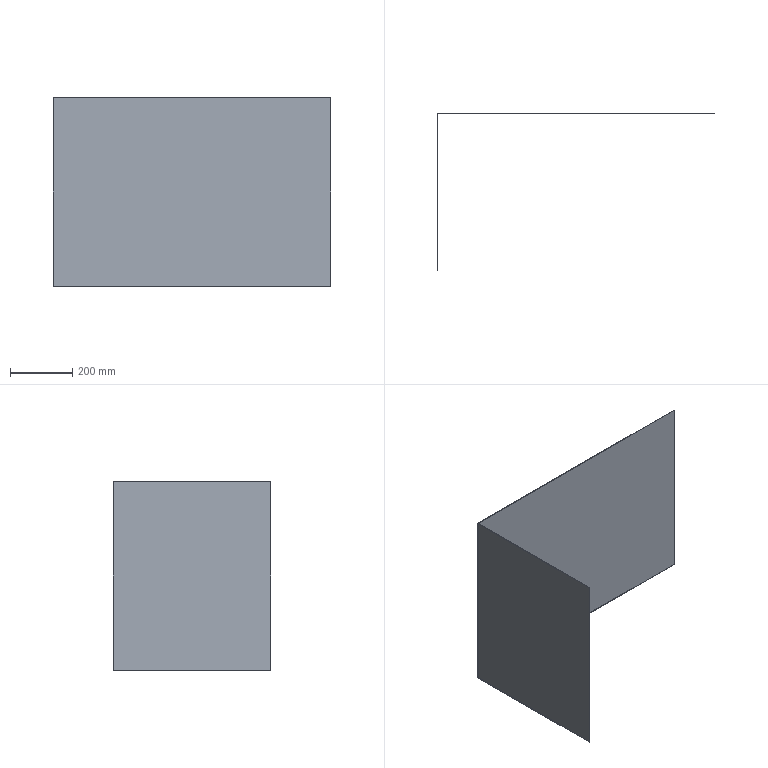Part | STEP file | zhi | 1 solid | 9 faces | box 891 x 505.5 x 606 mm | volume 845626 mm3 | plane 8 | cylinder 1 | commonest cylinder face diameters 1.2 x1
STEP:
#1=CARTESIAN_POINT('',(0.,0.,0.));
#2=DIRECTION('',(0.,0.,1.));
#3=DIRECTION('',(1.,0.,0.));
#4=AXIS2_PLACEMENT_3D('',#1,#2,#3);
#5=CARTESIAN_POINT('',(445.,-0.5,303.));
#6=VERTEX_POINT('',#5);
#7=CARTESIAN_POINT('',(445.,-0.5,-303.));
#8=VERTEX_POINT('',#7);
#9=CARTESIAN_POINT('',(445.,-0.5,-303.));
#10=DIRECTION('',(0.,0.,-1.));
#11=VECTOR('',#10,1.);
#12=LINE('',#9,#11);
#13=CARTESIAN_POINT('',(445.,0.5,-303.));
#14=DIRECTION('',(-1.,0.,0.));
#15=DIRECTION('',(0.,0.,1.));
#16=AXIS2_PLACEMENT_3D('',#13,#14,#15);
#17=PLANE('',#16);
#18=CARTESIAN_POINT('',(0.,-1.));
#19=DIRECTION('',(-1.,0.));
#20=VECTOR('',#19,1.);
#21=LINE('',#18,#20);
#22=(GEOMETRIC_REPRESENTATION_CONTEXT(2)PARAMETRIC_REPRESENTATION_CONTEXT()REPRESENTATION_CONTEXT('',''));
#23=DEFINITIONAL_REPRESENTATION('',(#21),#22);
#24=PCURVE('',#17,#23);
#25=CARTESIAN_POINT('',(0.,-0.5,0.));
#26=DIRECTION('',(0.,1.,0.));
#27=DIRECTION('',(0.,0.,1.));
#28=AXIS2_PLACEMENT_3D('',#25,#26,#27);
#29=PLANE('',#28);
#30=CARTESIAN_POINT('',(-303.,445.));
#31=DIRECTION('',(-1.,0.));
#32=VECTOR('',#31,1.);
#33=LINE('',#30,#32);
#34=(GEOMETRIC_REPRESENTATION_CONTEXT(2)PARAMETRIC_REPRESENTATION_CONTEXT()REPRESENTATION_CONTEXT('',''));
#35=DEFINITIONAL_REPRESENTATION('',(#33),#34);
#36=PCURVE('',#29,#35);
#37=SURFACE_CURVE('',#12,(#24,#36),.PCURVE_S1.);
#38=EDGE_CURVE('',#6,#8,#37,.T.);
#39=ORIENTED_EDGE('',*,*,#38,.T.);
#40=CARTESIAN_POINT('',(445.,0.5,-303.));
#41=VERTEX_POINT('',#40);
#42=CARTESIAN_POINT('',(445.,0.5,-303.));
#43=DIRECTION('',(0.,-1.,0.));
#44=VECTOR('',#43,1.);
#45=LINE('',#42,#44);
#46=CARTESIAN_POINT('',(0.,0.));
#47=DIRECTION('',(0.,-1.));
#48=VECTOR('',#47,1.);
#49=LINE('',#46,#48);
#50=(GEOMETRIC_REPRESENTATION_CONTEXT(2)PARAMETRIC_REPRESENTATION_CONTEXT()REPRESENTATION_CONTEXT('',''));
#51=DEFINITIONAL_REPRESENTATION('',(#49),#50);
#52=PCURVE('',#17,#51);
#53=CARTESIAN_POINT('',(-445.,0.5,-303.));
#54=DIRECTION('',(0.,0.,1.));
#55=DIRECTION('',(1.,0.,0.));
#56=AXIS2_PLACEMENT_3D('',#53,#54,#55);
#57=PLANE('',#56);
#58=CARTESIAN_POINT('',(890.,0.));
#59=DIRECTION('',(0.,-1.));
#60=VECTOR('',#59,1.);
#61=LINE('',#58,#60);
#62=(GEOMETRIC_REPRESENTATION_CONTEXT(2)PARAMETRIC_REPRESENTATION_CONTEXT()REPRESENTATION_CONTEXT('',''));
#63=DEFINITIONAL_REPRESENTATION('',(#61),#62);
#64=PCURVE('',#57,#63);
#65=SURFACE_CURVE('',#45,(#52,#64),.PCURVE_S1.);
#66=EDGE_CURVE('',#41,#8,#65,.T.);
#67=ORIENTED_EDGE('',*,*,#66,.F.);
#68=CARTESIAN_POINT('',(445.,0.5,303.));
#69=VERTEX_POINT('',#68);
#70=CARTESIAN_POINT('',(445.,0.5,-303.));
#71=DIRECTION('',(0.,0.,-1.));
#72=VECTOR('',#71,1.);
#73=LINE('',#70,#72);
#74=CARTESIAN_POINT('',(0.,0.));
#75=DIRECTION('',(-1.,0.));
#76=VECTOR('',#75,1.);
#77=LINE('',#74,#76);
#78=(GEOMETRIC_REPRESENTATION_CONTEXT(2)PARAMETRIC_REPRESENTATION_CONTEXT()REPRESENTATION_CONTEXT('',''));
#79=DEFINITIONAL_REPRESENTATION('',(#77),#78);
#80=PCURVE('',#17,#79);
#81=CARTESIAN_POINT('',(0.,0.5,0.));
#82=DIRECTION('',(0.,1.,0.));
#83=DIRECTION('',(0.,0.,1.));
#84=AXIS2_PLACEMENT_3D('',#81,#82,#83);
#85=PLANE('',#84);
#86=CARTESIAN_POINT('',(-303.,445.));
#87=DIRECTION('',(-1.,0.));
#88=VECTOR('',#87,1.);
#89=LINE('',#86,#88);
#90=(GEOMETRIC_REPRESENTATION_CONTEXT(2)PARAMETRIC_REPRESENTATION_CONTEXT()REPRESENTATION_CONTEXT('',''));
#91=DEFINITIONAL_REPRESENTATION('',(#89),#90);
#92=PCURVE('',#85,#91);
#93=SURFACE_CURVE('',#73,(#80,#92),.PCURVE_S1.);
#94=EDGE_CURVE('',#69,#41,#93,.T.);
#95=ORIENTED_EDGE('',*,*,#94,.F.);
#96=CARTESIAN_POINT('',(445.,0.5,303.));
#97=DIRECTION('',(0.,-1.,0.));
#98=VECTOR('',#97,1.);
#99=LINE('',#96,#98);
#100=CARTESIAN_POINT('',(606.,0.));
#101=DIRECTION('',(0.,-1.));
#102=VECTOR('',#101,1.);
#103=LINE('',#100,#102);
#104=(GEOMETRIC_REPRESENTATION_CONTEXT(2)PARAMETRIC_REPRESENTATION_CONTEXT()REPRESENTATION_CONTEXT('',''));
#105=DEFINITIONAL_REPRESENTATION('',(#103),#104);
#106=PCURVE('',#17,#105);
#107=CARTESIAN_POINT('',(-445.,0.5,303.));
#108=DIRECTION('',(0.,0.,-1.));
#109=DIRECTION('',(-1.,0.,0.));
#110=AXIS2_PLACEMENT_3D('',#107,#108,#109);
#111=PLANE('',#110);
#112=CARTESIAN_POINT('',(-890.,0.));
#113=DIRECTION('',(0.,-1.));
#114=VECTOR('',#113,1.);
#115=LINE('',#112,#114);
#116=(GEOMETRIC_REPRESENTATION_CONTEXT(2)PARAMETRIC_REPRESENTATION_CONTEXT()REPRESENTATION_CONTEXT('',''));
#117=DEFINITIONAL_REPRESENTATION('',(#115),#116);
#118=PCURVE('',#111,#117);
#119=SURFACE_CURVE('',#99,(#106,#118),.PCURVE_S1.);
#120=EDGE_CURVE('',#69,#6,#119,.T.);
#121=ORIENTED_EDGE('',*,*,#120,.T.);
#122=EDGE_LOOP('',(#39,#67,#95,#121));
#123=FACE_BOUND('',#122,.T.);
#124=ADVANCED_FACE('',(#123),#17,.F.);
#125=CARTESIAN_POINT('',(-446.,-0.1,-303.));
#126=VERTEX_POINT('',#125);
#127=CARTESIAN_POINT('',(-446.,-505.,-303.));
#128=VERTEX_POINT('',#127);
#129=CARTESIAN_POINT('',(-446.,0.5,-303.));
#130=DIRECTION('',(0.,-1.,0.));
#131=VECTOR('',#130,1.);
#132=LINE('',#129,#131);
#133=CARTESIAN_POINT('',(-1.,0.));
#134=DIRECTION('',(0.,-1.));
#135=VECTOR('',#134,1.);
#136=LINE('',#133,#135);
#137=(GEOMETRIC_REPRESENTATION_CONTEXT(2)PARAMETRIC_REPRESENTATION_CONTEXT()REPRESENTATION_CONTEXT('',''));
#138=DEFINITIONAL_REPRESENTATION('',(#136),#137);
#139=PCURVE('',#57,#138);
#140=CARTESIAN_POINT('',(-446.,0.,0.));
#141=DIRECTION('',(-1.,0.,0.));
#142=DIRECTION('',(0.,0.,1.));
#143=AXIS2_PLACEMENT_3D('',#140,#141,#142);
#144=PLANE('',#143);
#145=CARTESIAN_POINT('',(-303.,0.5));
#146=DIRECTION('',(0.,-1.));
#147=VECTOR('',#146,1.);
#148=LINE('',#145,#147);
#149=(GEOMETRIC_REPRESENTATION_CONTEXT(2)PARAMETRIC_REPRESENTATION_CONTEXT()REPRESENTATION_CONTEXT('',''));
#150=DEFINITIONAL_REPRESENTATION('',(#148),#149);
#151=PCURVE('',#144,#150);
#152=SURFACE_CURVE('',#132,(#139,#151),.PCURVE_S1.);
#153=EDGE_CURVE('',#126,#128,#152,.T.);
#154=ORIENTED_EDGE('',*,*,#153,.F.);
#155=CARTESIAN_POINT('',(-445.4,0.5,-303.));
#156=VERTEX_POINT('',#155);
#157=CARTESIAN_POINT('',(-445.4,-0.1,-303.));
#158=DIRECTION('',(0.,0.,-1.));
#159=DIRECTION('',(1.,0.,0.));
#160=AXIS2_PLACEMENT_3D('',#157,#158,#159);
#161=CIRCLE('',#160,0.6);
#162=CARTESIAN_POINT('',(0.2,-0.6));
#163=CARTESIAN_POINT('',(0.2,-1.639));
#164=CARTESIAN_POINT('',(-0.7,-1.12));
#165=CARTESIAN_POINT('',(-1.6,-0.6));
#166=CARTESIAN_POINT('',(-0.7,-0.08038));
#167=CARTESIAN_POINT('',(0.2,0.4392));
#168=CARTESIAN_POINT('',(0.2,-0.6));
#169=(BOUNDED_CURVE()B_SPLINE_CURVE(2,(#162,#163,#164,#165,#166,#167,#168),.UNSPECIFIED.,.T.,.F.)B_SPLINE_CURVE_WITH_KNOTS((1,2,2,2,2,1),(-2.094,0.,2.094,4.189,6.283,8.378),.UNSPECIFIED.)CURVE()GEOMETRIC_REPRESENTATION_ITEM()RATIONAL_B_SPLINE_CURVE((1.,0.5,1.,0.5,1.,0.5,1.))REPRESENTATION_ITEM(''));
#170=(GEOMETRIC_REPRESENTATION_CONTEXT(2)PARAMETRIC_REPRESENTATION_CONTEXT()REPRESENTATION_CONTEXT('',''));
#171=DEFINITIONAL_REPRESENTATION('',(#169),#170);
#172=PCURVE('',#57,#171);
#173=CARTESIAN_POINT('',(-445.4,-0.1,0.));
#174=DIRECTION('',(0.,0.,-1.));
#175=DIRECTION('',(-1.,0.,0.));
#176=AXIS2_PLACEMENT_3D('',#173,#174,#175);
#177=CYLINDRICAL_SURFACE('',#176,0.6);
#178=CARTESIAN_POINT('',(-3.142,303.));
#179=DIRECTION('',(1.,0.));
#180=VECTOR('',#179,1.);
#181=LINE('',#178,#180);
#182=(GEOMETRIC_REPRESENTATION_CONTEXT(2)PARAMETRIC_REPRESENTATION_CONTEXT()REPRESENTATION_CONTEXT('',''));
#183=DEFINITIONAL_REPRESENTATION('',(#181),#182);
#184=PCURVE('',#177,#183);
#185=SURFACE_CURVE('',#161,(#172,#184),.PCURVE_S1.);
#186=EDGE_CURVE('',#126,#156,#185,.T.);
#187=ORIENTED_EDGE('',*,*,#186,.T.);
#188=CARTESIAN_POINT('',(-445.,0.5,-303.));
#189=DIRECTION('',(-1.,0.,0.));
#190=VECTOR('',#189,1.);
#191=LINE('',#188,#190);
#192=CARTESIAN_POINT('',(0.,0.));
#193=DIRECTION('',(-1.,0.));
#194=VECTOR('',#193,1.);
#195=LINE('',#192,#194);
#196=(GEOMETRIC_REPRESENTATION_CONTEXT(2)PARAMETRIC_REPRESENTATION_CONTEXT()REPRESENTATION_CONTEXT('',''));
#197=DEFINITIONAL_REPRESENTATION('',(#195),#196);
#198=PCURVE('',#57,#197);
#199=CARTESIAN_POINT('',(-303.,-445.));
#200=DIRECTION('',(0.,-1.));
#201=VECTOR('',#200,1.);
#202=LINE('',#199,#201);
#203=(GEOMETRIC_REPRESENTATION_CONTEXT(2)PARAMETRIC_REPRESENTATION_CONTEXT()REPRESENTATION_CONTEXT('',''));
#204=DEFINITIONAL_REPRESENTATION('',(#202),#203);
#205=PCURVE('',#85,#204);
#206=SURFACE_CURVE('',#191,(#198,#205),.PCURVE_S1.);
#207=EDGE_CURVE('',#41,#156,#206,.T.);
#208=ORIENTED_EDGE('',*,*,#207,.F.);
#209=ORIENTED_EDGE('',*,*,#66,.T.);
#210=CARTESIAN_POINT('',(-445.,-0.5,-303.));
#211=VERTEX_POINT('',#210);
#212=CARTESIAN_POINT('',(-445.,-0.5,-303.));
#213=DIRECTION('',(-1.,0.,0.));
#214=VECTOR('',#213,1.);
#215=LINE('',#212,#214);
#216=CARTESIAN_POINT('',(0.,-1.));
#217=DIRECTION('',(-1.,0.));
#218=VECTOR('',#217,1.);
#219=LINE('',#216,#218);
#220=(GEOMETRIC_REPRESENTATION_CONTEXT(2)PARAMETRIC_REPRESENTATION_CONTEXT()REPRESENTATION_CONTEXT('',''));
#221=DEFINITIONAL_REPRESENTATION('',(#219),#220);
#222=PCURVE('',#57,#221);
#223=CARTESIAN_POINT('',(-303.,-445.));
#224=DIRECTION('',(0.,-1.));
#225=VECTOR('',#224,1.);
#226=LINE('',#223,#225);
#227=(GEOMETRIC_REPRESENTATION_CONTEXT(2)PARAMETRIC_REPRESENTATION_CONTEXT()REPRESENTATION_CONTEXT('',''));
#228=DEFINITIONAL_REPRESENTATION('',(#226),#227);
#229=PCURVE('',#29,#228);
#230=SURFACE_CURVE('',#215,(#222,#229),.PCURVE_S1.);
#231=EDGE_CURVE('',#8,#211,#230,.T.);
#232=ORIENTED_EDGE('',*,*,#231,.T.);
#233=CARTESIAN_POINT('',(-445.,-505.,-303.));
#234=VERTEX_POINT('',#233);
#235=CARTESIAN_POINT('',(-445.,0.5,-303.));
#236=DIRECTION('',(0.,-1.,0.));
#237=VECTOR('',#236,1.);
#238=LINE('',#235,#237);
#239=CARTESIAN_POINT('',(0.,0.));
#240=DIRECTION('',(0.,-1.));
#241=VECTOR('',#240,1.);
#242=LINE('',#239,#241);
#243=(GEOMETRIC_REPRESENTATION_CONTEXT(2)PARAMETRIC_REPRESENTATION_CONTEXT()REPRESENTATION_CONTEXT('',''));
#244=DEFINITIONAL_REPRESENTATION('',(#242),#243);
#245=PCURVE('',#57,#244);
#246=CARTESIAN_POINT('',(-445.,0.,0.));
#247=DIRECTION('',(-1.,0.,0.));
#248=DIRECTION('',(0.,0.,1.));
#249=AXIS2_PLACEMENT_3D('',#246,#247,#248);
#250=PLANE('',#249);
#251=CARTESIAN_POINT('',(-303.,0.5));
#252=DIRECTION('',(0.,-1.));
#253=VECTOR('',#252,1.);
#254=LINE('',#251,#253);
#255=(GEOMETRIC_REPRESENTATION_CONTEXT(2)PARAMETRIC_REPRESENTATION_CONTEXT()REPRESENTATION_CONTEXT('',''));
#256=DEFINITIONAL_REPRESENTATION('',(#254),#255);
#257=PCURVE('',#250,#256);
#258=SURFACE_CURVE('',#238,(#245,#257),.PCURVE_S1.);
#259=EDGE_CURVE('',#211,#234,#258,.T.);
#260=ORIENTED_EDGE('',*,*,#259,.T.);
#261=CARTESIAN_POINT('',(-446.,-505.,-303.));
#262=DIRECTION('',(1.,0.,0.));
#263=VECTOR('',#262,1.);
#264=LINE('',#261,#263);
#265=CARTESIAN_POINT('',(-1.,-505.5));
#266=DIRECTION('',(1.,0.));
#267=VECTOR('',#266,1.);
#268=LINE('',#265,#267);
#269=(GEOMETRIC_REPRESENTATION_CONTEXT(2)PARAMETRIC_REPRESENTATION_CONTEXT()REPRESENTATION_CONTEXT('',''));
#270=DEFINITIONAL_REPRESENTATION('',(#268),#269);
#271=PCURVE('',#57,#270);
#272=CARTESIAN_POINT('',(-446.,-505.,-303.));
#273=DIRECTION('',(0.,1.,0.));
#274=DIRECTION('',(0.,0.,1.));
#275=AXIS2_PLACEMENT_3D('',#272,#273,#274);
#276=PLANE('',#275);
#277=CARTESIAN_POINT('',(0.,0.));
#278=DIRECTION('',(0.,1.));
#279=VECTOR('',#278,1.);
#280=LINE('',#277,#279);
#281=(GEOMETRIC_REPRESENTATION_CONTEXT(2)PARAMETRIC_REPRESENTATION_CONTEXT()REPRESENTATION_CONTEXT('',''));
#282=DEFINITIONAL_REPRESENTATION('',(#280),#281);
#283=PCURVE('',#276,#282);
#284=SURFACE_CURVE('',#264,(#271,#283),.PCURVE_S1.);
#285=EDGE_CURVE('',#128,#234,#284,.T.);
#286=ORIENTED_EDGE('',*,*,#285,.F.);
#287=EDGE_LOOP('',(#154,#187,#208,#209,#232,#260,#286));
#288=FACE_BOUND('',#287,.T.);
#289=ADVANCED_FACE('',(#288),#57,.F.);
#290=CARTESIAN_POINT('',(-445.4,0.5,303.));
#291=VERTEX_POINT('',#290);
#292=CARTESIAN_POINT('',(-445.,0.5,303.));
#293=DIRECTION('',(1.,0.,0.));
#294=VECTOR('',#293,1.);
#295=LINE('',#292,#294);
#296=CARTESIAN_POINT('',(0.,0.));
#297=DIRECTION('',(-1.,0.));
#298=VECTOR('',#297,1.);
#299=LINE('',#296,#298);
#300=(GEOMETRIC_REPRESENTATION_CONTEXT(2)PARAMETRIC_REPRESENTATION_CONTEXT()REPRESENTATION_CONTEXT('',''));
#301=DEFINITIONAL_REPRESENTATION('',(#299),#300);
#302=PCURVE('',#111,#301);
#303=CARTESIAN_POINT('',(303.,-445.));
#304=DIRECTION('',(0.,1.));
#305=VECTOR('',#304,1.);
#306=LINE('',#303,#305);
#307=(GEOMETRIC_REPRESENTATION_CONTEXT(2)PARAMETRIC_REPRESENTATION_CONTEXT()REPRESENTATION_CONTEXT('',''));
#308=DEFINITIONAL_REPRESENTATION('',(#306),#307);
#309=PCURVE('',#85,#308);
#310=SURFACE_CURVE('',#295,(#302,#309),.PCURVE_S1.);
#311=EDGE_CURVE('',#291,#69,#310,.T.);
#312=ORIENTED_EDGE('',*,*,#311,.F.);
#313=CARTESIAN_POINT('',(-446.,-0.1,303.));
#314=VERTEX_POINT('',#313);
#315=CARTESIAN_POINT('',(-445.4,-0.1,303.));
#316=DIRECTION('',(0.,0.,1.));
#317=DIRECTION('',(-1.,0.,0.));
#318=AXIS2_PLACEMENT_3D('',#315,#316,#317);
#319=CIRCLE('',#318,0.6);
#320=CARTESIAN_POINT('',(1.,-0.6));
#321=CARTESIAN_POINT('',(1.,-1.639));
#322=CARTESIAN_POINT('',(0.1,-1.12));
#323=CARTESIAN_POINT('',(-0.8,-0.6));
#324=CARTESIAN_POINT('',(0.1,-0.08038));
#325=CARTESIAN_POINT('',(1.,0.4392));
#326=CARTESIAN_POINT('',(1.,-0.6));
#327=(BOUNDED_CURVE()B_SPLINE_CURVE(2,(#320,#321,#322,#323,#324,#325,#326),.UNSPECIFIED.,.T.,.F.)B_SPLINE_CURVE_WITH_KNOTS((1,2,2,2,2,1),(-2.094,0.,2.094,4.189,6.283,8.378),.UNSPECIFIED.)CURVE()GEOMETRIC_REPRESENTATION_ITEM()RATIONAL_B_SPLINE_CURVE((1.,0.5,1.,0.5,1.,0.5,1.))REPRESENTATION_ITEM(''));
#328=(GEOMETRIC_REPRESENTATION_CONTEXT(2)PARAMETRIC_REPRESENTATION_CONTEXT()REPRESENTATION_CONTEXT('',''));
#329=DEFINITIONAL_REPRESENTATION('',(#327),#328);
#330=PCURVE('',#111,#329);
#331=CARTESIAN_POINT('',(6.283,-303.));
#332=DIRECTION('',(-1.,0.));
#333=VECTOR('',#332,1.);
#334=LINE('',#331,#333);
#335=(GEOMETRIC_REPRESENTATION_CONTEXT(2)PARAMETRIC_REPRESENTATION_CONTEXT()REPRESENTATION_CONTEXT('',''));
#336=DEFINITIONAL_REPRESENTATION('',(#334),#335);
#337=PCURVE('',#177,#336);
#338=SURFACE_CURVE('',#319,(#330,#337),.PCURVE_S1.);
#339=EDGE_CURVE('',#291,#314,#338,.T.);
#340=ORIENTED_EDGE('',*,*,#339,.T.);
#341=CARTESIAN_POINT('',(-446.,-505.,303.));
#342=VERTEX_POINT('',#341);
#343=CARTESIAN_POINT('',(-446.,0.5,303.));
#344=DIRECTION('',(0.,1.,0.));
#345=VECTOR('',#344,1.);
#346=LINE('',#343,#345);
#347=CARTESIAN_POINT('',(1.,0.));
#348=DIRECTION('',(0.,1.));
#349=VECTOR('',#348,1.);
#350=LINE('',#347,#349);
#351=(GEOMETRIC_REPRESENTATION_CONTEXT(2)PARAMETRIC_REPRESENTATION_CONTEXT()REPRESENTATION_CONTEXT('',''));
#352=DEFINITIONAL_REPRESENTATION('',(#350),#351);
#353=PCURVE('',#111,#352);
#354=CARTESIAN_POINT('',(303.,0.5));
#355=DIRECTION('',(0.,1.));
#356=VECTOR('',#355,1.);
#357=LINE('',#354,#356);
#358=(GEOMETRIC_REPRESENTATION_CONTEXT(2)PARAMETRIC_REPRESENTATION_CONTEXT()REPRESENTATION_CONTEXT('',''));
#359=DEFINITIONAL_REPRESENTATION('',(#357),#358);
#360=PCURVE('',#144,#359);
#361=SURFACE_CURVE('',#346,(#353,#360),.PCURVE_S1.);
#362=EDGE_CURVE('',#342,#314,#361,.T.);
#363=ORIENTED_EDGE('',*,*,#362,.F.);
#364=CARTESIAN_POINT('',(-445.,-505.,303.));
#365=VERTEX_POINT('',#364);
#366=CARTESIAN_POINT('',(-446.,-505.,303.));
#367=DIRECTION('',(1.,0.,0.));
#368=VECTOR('',#367,1.);
#369=LINE('',#366,#368);
#370=CARTESIAN_POINT('',(1.,-505.5));
#371=DIRECTION('',(-1.,0.));
#372=VECTOR('',#371,1.);
#373=LINE('',#370,#372);
#374=(GEOMETRIC_REPRESENTATION_CONTEXT(2)PARAMETRIC_REPRESENTATION_CONTEXT()REPRESENTATION_CONTEXT('',''));
#375=DEFINITIONAL_REPRESENTATION('',(#373),#374);
#376=PCURVE('',#111,#375);
#377=CARTESIAN_POINT('',(606.,0.));
#378=DIRECTION('',(0.,1.));
#379=VECTOR('',#378,1.);
#380=LINE('',#377,#379);
#381=(GEOMETRIC_REPRESENTATION_CONTEXT(2)PARAMETRIC_REPRESENTATION_CONTEXT()REPRESENTATION_CONTEXT('',''));
#382=DEFINITIONAL_REPRESENTATION('',(#380),#381);
#383=PCURVE('',#276,#382);
#384=SURFACE_CURVE('',#369,(#376,#383),.PCURVE_S1.);
#385=EDGE_CURVE('',#342,#365,#384,.T.);
#386=ORIENTED_EDGE('',*,*,#385,.T.);
#387=CARTESIAN_POINT('',(-445.,-0.5,303.));
#388=VERTEX_POINT('',#387);
#389=CARTESIAN_POINT('',(-445.,0.5,303.));
#390=DIRECTION('',(0.,1.,0.));
#391=VECTOR('',#390,1.);
#392=LINE('',#389,#391);
#393=CARTESIAN_POINT('',(0.,0.));
#394=DIRECTION('',(0.,1.));
#395=VECTOR('',#394,1.);
#396=LINE('',#393,#395);
#397=(GEOMETRIC_REPRESENTATION_CONTEXT(2)PARAMETRIC_REPRESENTATION_CONTEXT()REPRESENTATION_CONTEXT('',''));
#398=DEFINITIONAL_REPRESENTATION('',(#396),#397);
#399=PCURVE('',#111,#398);
#400=CARTESIAN_POINT('',(303.,0.5));
#401=DIRECTION('',(0.,1.));
#402=VECTOR('',#401,1.);
#403=LINE('',#400,#402);
#404=(GEOMETRIC_REPRESENTATION_CONTEXT(2)PARAMETRIC_REPRESENTATION_CONTEXT()REPRESENTATION_CONTEXT('',''));
#405=DEFINITIONAL_REPRESENTATION('',(#403),#404);
#406=PCURVE('',#250,#405);
#407=SURFACE_CURVE('',#392,(#399,#406),.PCURVE_S1.);
#408=EDGE_CURVE('',#365,#388,#407,.T.);
#409=ORIENTED_EDGE('',*,*,#408,.T.);
#410=CARTESIAN_POINT('',(-445.,-0.5,303.));
#411=DIRECTION('',(1.,0.,0.));
#412=VECTOR('',#411,1.);
#413=LINE('',#410,#412);
#414=CARTESIAN_POINT('',(0.,-1.));
#415=DIRECTION('',(-1.,0.));
#416=VECTOR('',#415,1.);
#417=LINE('',#414,#416);
#418=(GEOMETRIC_REPRESENTATION_CONTEXT(2)PARAMETRIC_REPRESENTATION_CONTEXT()REPRESENTATION_CONTEXT('',''));
#419=DEFINITIONAL_REPRESENTATION('',(#417),#418);
#420=PCURVE('',#111,#419);
#421=CARTESIAN_POINT('',(303.,-445.));
#422=DIRECTION('',(0.,1.));
#423=VECTOR('',#422,1.);
#424=LINE('',#421,#423);
#425=(GEOMETRIC_REPRESENTATION_CONTEXT(2)PARAMETRIC_REPRESENTATION_CONTEXT()REPRESENTATION_CONTEXT('',''));
#426=DEFINITIONAL_REPRESENTATION('',(#424),#425);
#427=PCURVE('',#29,#426);
#428=SURFACE_CURVE('',#413,(#420,#427),.PCURVE_S1.);
#429=EDGE_CURVE('',#388,#6,#428,.T.);
#430=ORIENTED_EDGE('',*,*,#429,.T.);
#431=ORIENTED_EDGE('',*,*,#120,.F.);
#432=EDGE_LOOP('',(#312,#340,#363,#386,#409,#430,#431));
#433=FACE_BOUND('',#432,.T.);
#434=ADVANCED_FACE('',(#433),#111,.F.);
#435=ORIENTED_EDGE('',*,*,#207,.T.);
#436=CARTESIAN_POINT('',(-445.4,0.5,0.));
#437=DIRECTION('',(0.,0.,1.));
#438=VECTOR('',#437,1.);
#439=LINE('',#436,#438);
#440=CARTESIAN_POINT('',(0.,-445.4));
#441=DIRECTION('',(1.,0.));
#442=VECTOR('',#441,1.);
#443=LINE('',#440,#442);
#444=(GEOMETRIC_REPRESENTATION_CONTEXT(2)PARAMETRIC_REPRESENTATION_CONTEXT()REPRESENTATION_CONTEXT('',''));
#445=DEFINITIONAL_REPRESENTATION('',(#443),#444);
#446=PCURVE('',#85,#445);
#447=CARTESIAN_POINT('',(1.571,0.));
#448=DIRECTION('',(0.,-1.));
#449=VECTOR('',#448,1.);
#450=LINE('',#447,#449);
#451=(GEOMETRIC_REPRESENTATION_CONTEXT(2)PARAMETRIC_REPRESENTATION_CONTEXT()REPRESENTATION_CONTEXT('',''));
#452=DEFINITIONAL_REPRESENTATION('',(#450),#451);
#453=PCURVE('',#177,#452);
#454=SURFACE_CURVE('',#439,(#446,#453),.PCURVE_S1.);
#455=EDGE_CURVE('',#156,#291,#454,.T.);
#456=ORIENTED_EDGE('',*,*,#455,.T.);
#457=ORIENTED_EDGE('',*,*,#311,.T.);
#458=ORIENTED_EDGE('',*,*,#94,.T.);
#459=EDGE_LOOP('',(#435,#456,#457,#458));
#460=FACE_BOUND('',#459,.T.);
#461=ADVANCED_FACE('',(#460),#85,.T.);
#462=ORIENTED_EDGE('',*,*,#38,.F.);
#463=ORIENTED_EDGE('',*,*,#429,.F.);
#464=CARTESIAN_POINT('',(-445.,-0.5,-303.));
#465=DIRECTION('',(0.,0.,1.));
#466=VECTOR('',#465,1.);
#467=LINE('',#464,#466);
#468=CARTESIAN_POINT('',(-303.,-445.));
#469=DIRECTION('',(1.,0.));
#470=VECTOR('',#469,1.);
#471=LINE('',#468,#470);
#472=(GEOMETRIC_REPRESENTATION_CONTEXT(2)PARAMETRIC_REPRESENTATION_CONTEXT()REPRESENTATION_CONTEXT('',''));
#473=DEFINITIONAL_REPRESENTATION('',(#471),#472);
#474=PCURVE('',#29,#473);
#475=CARTESIAN_POINT('',(-303.,-0.5));
#476=DIRECTION('',(1.,0.));
#477=VECTOR('',#476,1.);
#478=LINE('',#475,#477);
#479=(GEOMETRIC_REPRESENTATION_CONTEXT(2)PARAMETRIC_REPRESENTATION_CONTEXT()REPRESENTATION_CONTEXT('',''));
#480=DEFINITIONAL_REPRESENTATION('',(#478),#479);
#481=PCURVE('',#250,#480);
#482=SURFACE_CURVE('',#467,(#474,#481),.PCURVE_S1.);
#483=EDGE_CURVE('',#211,#388,#482,.T.);
#484=ORIENTED_EDGE('',*,*,#483,.F.);
#485=ORIENTED_EDGE('',*,*,#231,.F.);
#486=EDGE_LOOP('',(#462,#463,#484,#485));
#487=FACE_BOUND('',#486,.T.);
#488=ADVANCED_FACE('',(#487),#29,.F.);
#489=ORIENTED_EDGE('',*,*,#259,.F.);
#490=ORIENTED_EDGE('',*,*,#483,.T.);
#491=ORIENTED_EDGE('',*,*,#408,.F.);
#492=CARTESIAN_POINT('',(-445.,-505.,-303.));
#493=DIRECTION('',(0.,0.,1.));
#494=VECTOR('',#493,1.);
#495=LINE('',#492,#494);
#496=CARTESIAN_POINT('',(-303.,-505.));
#497=DIRECTION('',(1.,0.));
#498=VECTOR('',#497,1.);
#499=LINE('',#496,#498);
#500=(GEOMETRIC_REPRESENTATION_CONTEXT(2)PARAMETRIC_REPRESENTATION_CONTEXT()REPRESENTATION_CONTEXT('',''));
#501=DEFINITIONAL_REPRESENTATION('',(#499),#500);
#502=PCURVE('',#250,#501);
#503=CARTESIAN_POINT('',(0.,1.));
#504=DIRECTION('',(1.,0.));
#505=VECTOR('',#504,1.);
#506=LINE('',#503,#505);
#507=(GEOMETRIC_REPRESENTATION_CONTEXT(2)PARAMETRIC_REPRESENTATION_CONTEXT()REPRESENTATION_CONTEXT('',''));
#508=DEFINITIONAL_REPRESENTATION('',(#506),#507);
#509=PCURVE('',#276,#508);
#510=SURFACE_CURVE('',#495,(#502,#509),.PCURVE_S1.);
#511=EDGE_CURVE('',#234,#365,#510,.T.);
#512=ORIENTED_EDGE('',*,*,#511,.F.);
#513=EDGE_LOOP('',(#489,#490,#491,#512));
#514=FACE_BOUND('',#513,.T.);
#515=ADVANCED_FACE('',(#514),#250,.F.);
#516=ORIENTED_EDGE('',*,*,#511,.T.);
#517=ORIENTED_EDGE('',*,*,#385,.F.);
#518=CARTESIAN_POINT('',(-446.,-505.,-303.));
#519=DIRECTION('',(0.,0.,1.));
#520=VECTOR('',#519,1.);
#521=LINE('',#518,#520);
#522=CARTESIAN_POINT('',(0.,0.));
#523=DIRECTION('',(1.,0.));
#524=VECTOR('',#523,1.);
#525=LINE('',#522,#524);
#526=(GEOMETRIC_REPRESENTATION_CONTEXT(2)PARAMETRIC_REPRESENTATION_CONTEXT()REPRESENTATION_CONTEXT('',''));
#527=DEFINITIONAL_REPRESENTATION('',(#525),#526);
#528=PCURVE('',#276,#527);
#529=CARTESIAN_POINT('',(-303.,-505.));
#530=DIRECTION('',(1.,0.));
#531=VECTOR('',#530,1.);
#532=LINE('',#529,#531);
#533=(GEOMETRIC_REPRESENTATION_CONTEXT(2)PARAMETRIC_REPRESENTATION_CONTEXT()REPRESENTATION_CONTEXT('',''));
#534=DEFINITIONAL_REPRESENTATION('',(#532),#533);
#535=PCURVE('',#144,#534);
#536=SURFACE_CURVE('',#521,(#528,#535),.PCURVE_S1.);
#537=EDGE_CURVE('',#128,#342,#536,.T.);
#538=ORIENTED_EDGE('',*,*,#537,.F.);
#539=ORIENTED_EDGE('',*,*,#285,.T.);
#540=EDGE_LOOP('',(#516,#517,#538,#539));
#541=FACE_BOUND('',#540,.T.);
#542=ADVANCED_FACE('',(#541),#276,.F.);
#543=ORIENTED_EDGE('',*,*,#362,.T.);
#544=CARTESIAN_POINT('',(-446.,-0.1,0.));
#545=DIRECTION('',(0.,0.,-1.));
#546=VECTOR('',#545,1.);
#547=LINE('',#544,#546);
#548=CARTESIAN_POINT('',(0.,-0.1));
#549=DIRECTION('',(-1.,0.));
#550=VECTOR('',#549,1.);
#551=LINE('',#548,#550);
#552=(GEOMETRIC_REPRESENTATION_CONTEXT(2)PARAMETRIC_REPRESENTATION_CONTEXT()REPRESENTATION_CONTEXT('',''));
#553=DEFINITIONAL_REPRESENTATION('',(#551),#552);
#554=PCURVE('',#144,#553);
#555=CARTESIAN_POINT('',(0.,0.));
#556=DIRECTION('',(0.,1.));
#557=VECTOR('',#556,1.);
#558=LINE('',#555,#557);
#559=(GEOMETRIC_REPRESENTATION_CONTEXT(2)PARAMETRIC_REPRESENTATION_CONTEXT()REPRESENTATION_CONTEXT('',''));
#560=DEFINITIONAL_REPRESENTATION('',(#558),#559);
#561=PCURVE('',#177,#560);
#562=SURFACE_CURVE('',#547,(#554,#561),.PCURVE_S1.);
#563=EDGE_CURVE('',#314,#126,#562,.T.);
#564=ORIENTED_EDGE('',*,*,#563,.T.);
#565=ORIENTED_EDGE('',*,*,#153,.T.);
#566=ORIENTED_EDGE('',*,*,#537,.T.);
#567=EDGE_LOOP('',(#543,#564,#565,#566));
#568=FACE_BOUND('',#567,.T.);
#569=ADVANCED_FACE('',(#568),#144,.T.);
#570=ORIENTED_EDGE('',*,*,#339,.F.);
#571=ORIENTED_EDGE('',*,*,#455,.F.);
#572=ORIENTED_EDGE('',*,*,#186,.F.);
#573=ORIENTED_EDGE('',*,*,#563,.F.);
#574=EDGE_LOOP('',(#570,#571,#572,#573));
#575=FACE_BOUND('',#574,.T.);
#576=ADVANCED_FACE('',(#575),#177,.T.);
#577=CLOSED_SHELL('',(#124,#289,#434,#461,#488,#515,#542,#569,#576));
#578=MANIFOLD_SOLID_BREP('',#577);
#579=(LENGTH_UNIT()NAMED_UNIT(*)SI_UNIT(.MILLI.,.METRE.));
#580=UNCERTAINTY_MEASURE_WITH_UNIT(LENGTH_MEASURE(0.0000001),#579,'','');
#581=(NAMED_UNIT(*)PLANE_ANGLE_UNIT()SI_UNIT($,.RADIAN.));
#582=(NAMED_UNIT(*)SI_UNIT($,.STERADIAN.)SOLID_ANGLE_UNIT());
#583=(GEOMETRIC_REPRESENTATION_CONTEXT(3)GLOBAL_UNCERTAINTY_ASSIGNED_CONTEXT((#580))GLOBAL_UNIT_ASSIGNED_CONTEXT((#579,#581,#582))REPRESENTATION_CONTEXT('',''));
#584=ADVANCED_BREP_SHAPE_REPRESENTATION('',(#4,#578),#583);